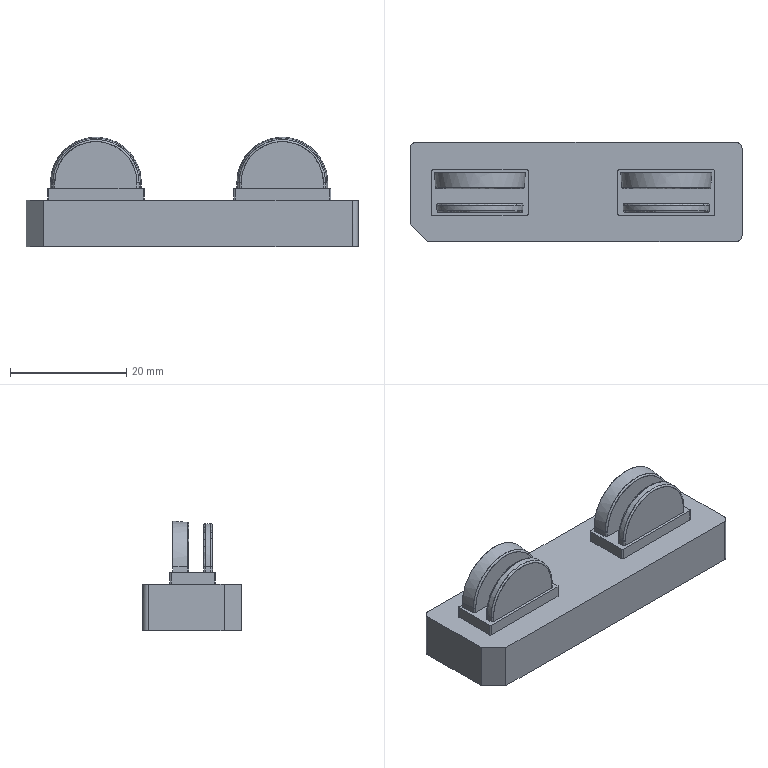NC program | PowerMill | posted by the shop | part box 57 x 17 x 18.807 mm
Lines 22103 to 22893 of 381081:
( TOOL ID   D10_1_1_1 )
( TOOL DIA. 10. TIP RAD 0 LENGTH 73.96 )
( Z = -11.01 )
T3 M6
T4
G91 G28 Z0
G0 G90 G54
M08
S8500 M3
X0 Y0 M8
G43 Z9.797 H3
X27.887 Y19.247
Z-9.81
G1 Z-11.01 F360
X27.699 Y13.975 F600
X18.085 Y9.168
X23.607
X23.828 Y9.163
X24.048 Y9.15
G2 X24.589 Y9.08 I-.615 J-6.925
G1 X24.858 Y9.026
G2 X26.347 Y8.449 I-1.315 J-5.601
G1 X26.555 Y8.325
G2 X27.127 Y7.914 I-3.108 J-4.931
G1 X27.189 Y7.865
X27.374 Y7.704
X27.552 Y7.534
X27.722 Y7.355
X27.884 Y7.17
X28.07 Y6.934
X28.211 Y6.738
X28.344 Y6.536
X28.467 Y6.329
X28.581 Y6.115
G2 X28.799 Y5.626 I-5.64 J-2.807
G1 X28.894 Y5.368
X28.976 Y5.106
X29.044 Y4.84
G2 X29.168 Y4.03 I-6.042 J-1.34
G1 X29.182 Y3.809
X29.187 Y3.588
Y-3.824
X29.182 Y-4.045
X29.168 Y-4.266
X29.14 Y-4.534
X29.099 Y-4.806
X29.044 Y-5.076
X28.976 Y-5.342
X28.894 Y-5.604
X28.78 Y-5.911
X28.685 Y-6.134
X28.581 Y-6.351
X28.467 Y-6.564
X28.344 Y-6.772
G2 X28.037 Y-7.214 I-5.063 J3.195
G1 X27.884 Y-7.406
X27.722 Y-7.592
G2 X27.374 Y-7.94 I-4.45 J4.102
G1 X27.189 Y-8.101
G2 X26.555 Y-8.561 I-3.982 J4.821
G1 X26.347 Y-8.685
X26.134 Y-8.799
X25.916 Y-8.903
G2 X25.387 Y-9.112 I-2.782 J6.274
G1 X25.124 Y-9.193
X24.858 Y-9.262
X24.589 Y-9.316
X24.268 Y-9.363
G2 X23.607 Y-9.404 I-.677 J5.595
G1 X7.393
G2 X6.527 Y-9.334 I.012 J5.527
G1 X6.411 Y-9.316
X6.142 Y-9.262
X5.876 Y-9.194
X5.613 Y-9.112
X5.306 Y-8.997
G2 X4.004 Y-8.254 I2.033 J5.076
G1 X3.811 Y-8.101
G2 X3.448 Y-7.77 I3.851 J4.585
X3.116 Y-7.406 I4.292 J4.249
X2.759 Y-6.929 I4.814 J3.975
G1 X2.656 Y-6.772
X2.539 Y-6.576
G2 X2.201 Y-5.862 I4.876 J2.751
G1 X2.106 Y-5.604
X2.024 Y-5.342
X1.956 Y-5.076
X1.901 Y-4.806
X1.86 Y-4.534
G2 X1.813 Y-3.824 I5.658 J.73
G1 Y3.588
X1.817 Y3.773
X1.838 Y4.104
X1.86 Y4.298
X1.901 Y4.57
X1.956 Y4.84
X2.024 Y5.106
X2.106 Y5.368
X2.22 Y5.675
X2.315 Y5.897
X2.419 Y6.116
X2.533 Y6.328
X2.656 Y6.536
G2 X2.97 Y6.987 I4.948 J-3.118
G1 X3.116 Y7.17
X3.278 Y7.356
X3.448 Y7.533
X3.626 Y7.704
G2 X4.033 Y8.04 I3.98 J-4.401
G1 X4.243 Y8.193
X4.445 Y8.325
X4.653 Y8.448
X4.866 Y8.563
X5.084 Y8.667
X5.27 Y8.746
X5.613 Y8.876
X5.876 Y8.958
X6.142 Y9.026
X6.411 Y9.08
X6.683 Y9.121
G2 X7.393 Y9.168 I.726 J-5.596
G1 X18.085
G0 Z2.804
G1 X1.885 Y4.466 F10000
G0 Z-10.91
G1 X1.86 Y4.298 Z-10.913 F360
X1.856 Y4.268
X1.854 Y4.25 Z-10.914
X1.827 Y3.959 Z-10.919
X1.813 Y3.588 Z-10.925
Y-1.26 Z-11.01
X-2.956 Y4.84 F600
X-2.901 Y4.57
X-2.854 Y4.25
X-2.832 Y4.03
X-2.818 Y3.809
X-2.813 Y3.588
Y-3.824
G2 X-2.854 Y-4.486 I-5.523 J.009
G1 X-2.901 Y-4.806
X-2.956 Y-5.076
X-3.024 Y-5.342
X-3.106 Y-5.604
X-3.22 Y-5.911
X-3.315 Y-6.134
X-3.419 Y-6.351
X-3.533 Y-6.564
X-3.656 Y-6.772
G2 X-3.963 Y-7.214 I-5.076 J3.204
G1 X-4.116 Y-7.406
X-4.278 Y-7.592
X-4.448 Y-7.769
X-4.626 Y-7.94
X-4.811 Y-8.101
G2 X-5.445 Y-8.561 I-4.018 J4.871
G1 X-5.653 Y-8.685
X-5.866 Y-8.798
X-6.084 Y-8.903
X-6.355 Y-9.017
X-6.613 Y-9.112
G2 X-7.142 Y-9.262 I-1.945 J5.846
G1 X-7.411 Y-9.316
X-7.683 Y-9.357
G2 X-8.172 Y-9.399 I-.745 J5.768
G1 X-8.393 Y-9.404
X-24.607
G2 X-25.95 Y-9.238 I.02 J5.69
G1 X-26.124 Y-9.193
G2 X-26.694 Y-8.997 I1.779 J6.081
G1 X-26.916 Y-8.903
G2 X-27.757 Y-8.429 I2.29 J5.043
G1 X-27.953 Y-8.287
G2 X-28.552 Y-7.77 I3.474 J4.631
G1 X-28.722 Y-7.592
G2 X-29.344 Y-6.772 I4.472 J4.038
G1 X-29.467 Y-6.564
X-29.581 Y-6.351
X-29.685 Y-6.134
X-29.793 Y-5.877
X-29.914 Y-5.542
X-29.976 Y-5.342
X-30.045 Y-5.075
X-30.099 Y-4.806
X-30.14 Y-4.534
G2 X-30.182 Y-4.045 I5.737 J.743
G1 X-30.187 Y-3.824
Y3.588
X-30.182 Y3.809
X-30.168 Y4.03
X-30.14 Y4.298
X-30.099 Y4.57
X-30.044 Y4.84
X-29.976 Y5.106
X-29.894 Y5.368
G2 X-29.685 Y5.898 I6.529 J-2.272
G1 X-29.581 Y6.115
X-29.467 Y6.329
X-29.343 Y6.536
X-29.211 Y6.738
G2 X-28.884 Y7.17 I5.641 J-3.936
G1 X-28.722 Y7.356
X-28.552 Y7.534
X-28.374 Y7.703
X-28.189 Y7.865
G2 X-27.555 Y8.325 I3.947 J-4.773
G1 X-27.347 Y8.449
X-27.134 Y8.562
X-26.916 Y8.667
X-26.645 Y8.781
X-26.387 Y8.876
G2 X-25.589 Y9.08 I1.818 J-5.43
G1 X-25.268 Y9.127
X-25.048 Y9.15
X-24.828 Y9.163
X-24.607 Y9.168
X-8.393
G2 X-7.079 Y9.01 I-.021 J-5.714
G1 X-6.876 Y8.957
G2 X-5.866 Y8.563 I-1.668 J-5.753
G1 X-5.653 Y8.449
X-5.445 Y8.325
G2 X-4.854 Y7.899 I-3.174 J-5.028
G1 X-4.626 Y7.704
X-4.448 Y7.534
X-4.278 Y7.356
X-4.116 Y7.17
X-3.93 Y6.934
X-3.789 Y6.738
X-3.656 Y6.536
G2 X-3.292 Y5.845 I-4.609 J-2.867
G1 X-3.201 Y5.626
X-3.106 Y5.368
X-3.024 Y5.106
X-2.956 Y4.84
G0 Z9.797
Z10.797
X0 Y0
X-4.092 Y-7.636
Z-9.78
G1 Z-10.98 F360
G3 X-5.2 Y-7.939 I-.188 J-1.488 F600
G2 X-8.306 Y-9.033 I-3.196 J4.117
G1 X-16.521 Y-9.034
X-24.555
G2 X-29.817 Y-3.834 I-.05 J5.212
G1 X-29.816 Y3.654
G2 X-24.554 Y8.798 I5.212 J-.068
G1 X-8.303 Y8.797
G2 X-3.184 Y3.651 I-.092 J-5.211
G1 X-3.183 Y-3.835
G2 X-5.2 Y-7.939 I-5.212 J.013
G3 X-5.768 Y-8.937 I.92 J-1.185
G1 X-4.16 Y-7.594
G3 X-5.269 Y-7.892 I-.195 J-1.487
G2 X-8.489 Y-8.954 I-3.128 J4.071
G1 X-16.521
X-24.554
X-24.555
G2 X-29.737 Y-3.834 I-.049 J5.132
G1 X-29.736 Y3.651
G2 X-24.554 Y8.718 I5.132 J-.065
G1 X-8.489
G2 X-3.264 Y3.651 I.091 J-5.133
G1 X-3.263 Y-3.834
G2 X-5.269 Y-7.892 I-5.134 J.013
G3 X-5.843 Y-8.886 I.914 J-1.189
G0 Z3.9
G1 X27.901 Y-7.644 F10000
G0 Z-9.78
G1 Z-10.98 F360
G3 X26.793 Y-7.945 I-.19 J-1.488 F600
G2 X23.641 Y-9.034 I-3.188 J4.123
G1 X7.392
G2 X2.268 Y-4.759 I.003 J5.211
G1 X2.251 Y-4.658
G2 X2.183 Y-3.834 I5.297 J.849
G1 Y-3.118
X2.184 Y3.654
G2 X7.394 Y8.798 I5.211 J-.067
G1 X23.643
G2 X28.816 Y3.651 I-.038 J-5.212
G1 X28.817 Y-3.835
G2 X26.793 Y-7.945 I-5.212 J.013
G3 X26.223 Y-8.942 I.918 J-1.187
G1 X27.833 Y-7.602
G3 X26.724 Y-7.898 I-.198 J-1.487
G2 X23.641 Y-8.954 I-3.119 J4.075
G1 X7.394
G2 X2.347 Y-4.746 I.001 J5.131
G1 X2.33 Y-4.645
G2 X2.263 Y-3.834 I5.216 J.836
G1 Y-3.118
X2.264 Y3.651
G2 X7.394 Y8.718 I5.131 J-.065
G1 X23.641
G2 X28.736 Y3.651 I-.036 J-5.132
G1 X28.737 Y-3.834
G2 X26.724 Y-7.898 I-5.132 J.011
G3 X26.148 Y-8.891 I.912 J-1.191
G0 Z10.797
X0 Y0
Z9.797
X32.183 Y-17.539
Z-17.71
G1 Z-18.91 F360
G3 X30.071 Y-13.007 I-1.056 J2.266 F600
G1 X29.91 Y-13.082
X29.907 Y-13.083
X29.905 Y-13.084
X29.589 Y-13.21
X29.587 Y-13.211
X29.585
X29.269 Y-13.317
X29.267
X29.266 Y-13.318
X29.139 Y-13.355
X29.138
X29.137 Y-13.356
X28.948 Y-13.405
X28.946 Y-13.406
X28.944
X28.628 Y-13.474
X28.626 Y-13.475
X28.624
X28.308 Y-13.526
X28.306
X28.303 Y-13.527
X27.987 Y-13.56
X27.985
X27.983
X27.667 Y-13.577
X27.665
X27.663
X27.347 Y-13.58
X-25.45
X-25.451
X-25.452
X-25.768 Y-13.573
X-25.77
X-25.773
X-26.089 Y-13.546
X-26.091 Y-13.545
X-26.094
X-26.41 Y-13.498
X-26.413 Y-13.497
X-26.415
X-26.731 Y-13.429
X-26.734 Y-13.428
X-26.736 Y-13.427
X-26.994 Y-13.355
X-26.997 Y-13.354
X-27.
X-27.373 Y-13.222
X-27.376 Y-13.221
X-27.379 Y-13.22
X-27.695 Y-13.081
X-27.696
X-27.698 Y-13.08
X-27.792 Y-13.034
X-27.793 Y-13.033
X-27.794 Y-13.032
X-28.017 Y-12.913
X-28.019 Y-12.911
X-28.021 Y-12.91
X-28.337 Y-12.714
X-28.34 Y-12.712
X-28.342 Y-12.71
X-28.658 Y-12.479
X-28.66 Y-12.477
X-28.662 Y-12.476
X-28.765 Y-12.392
X-28.766 Y-12.391
X-28.768 Y-12.389
X-28.98 Y-12.2
X-28.982 Y-12.199
X-28.983 Y-12.198
X-29.113 Y-12.071
X-29.114 Y-12.07
X-32.145 Y-9.038
X-32.146 Y-9.037
X-32.147 Y-9.036
X-32.268 Y-8.907
X-32.27 Y-8.905
X-32.271 Y-8.904
X-32.466 Y-8.675
X-32.467 Y-8.673
X-32.468 Y-8.672
X-32.536 Y-8.585
X-32.537 Y-8.584
X-32.538 Y-8.582
X-32.761 Y-8.266
X-32.763 Y-8.263
X-32.764 Y-8.261
X-32.953 Y-7.945
X-32.954 Y-7.942
X-32.956 Y-7.94
X-33.109 Y-7.637
X-33.11 Y-7.634
X-33.111 Y-7.632
X-33.249 Y-7.302
X-33.251 Y-7.3
Y-7.297
X-33.359 Y-6.981
X-33.36 Y-6.979
X-33.361 Y-6.976
X-33.43 Y-6.723
X-33.431 Y-6.721
X-33.432 Y-6.718
X-33.51 Y-6.339
X-33.511 Y-6.336
Y-6.334
X-33.554 Y-6.017
Y-6.015
Y-6.012
X-33.576 Y-5.696
Y-5.694
Y-5.692
X-33.58 Y-5.375
Y-5.374
X-33.579 Y7.588
Y7.589
Y7.591
X-33.566 Y7.907
Y7.909
Y7.911
X-33.536 Y8.227
Y8.229
Y8.231
X-33.489 Y8.548
Y8.55
X-33.488 Y8.552
X-33.432 Y8.834
X-33.431 Y8.836
Y8.838
X-33.341 Y9.188
X-33.34 Y9.19
Y9.193
X-33.238 Y9.509
Y9.511
X-33.237 Y9.513
X-33.116 Y9.829
X-33.115 Y9.831
X-33.114 Y9.833
X-32.972 Y10.149
X-32.971 Y10.152
X-32.97 Y10.154
X-32.805 Y10.47
X-32.804 Y10.472
X-32.803 Y10.474
X-32.613 Y10.79
X-32.612 Y10.792
X-32.61 Y10.794
X-32.471 Y11.
Y11.001
X-32.47 Y11.003
X-32.391 Y11.112
X-32.39 Y11.113
X-32.389 Y11.115
X-32.152 Y11.415
X-32.15 Y11.417
X-32.148 Y11.419
X-31.847 Y11.751
X-31.844 Y11.753
X-31.842 Y11.755
X-31.511 Y12.069
X-31.509 Y12.071
X-31.507 Y12.072
X-31.191 Y12.331
X-31.19 Y12.332
X-31.188 Y12.333
X-31.108 Y12.394
X-31.107 Y12.395
X-31.106
X-30.87 Y12.56
X-30.868 Y12.561
X-30.867 Y12.562
X-30.55 Y12.759
X-30.548 Y12.761
X-30.546 Y12.762
X-30.23 Y12.933
X-30.228 Y12.934
X-30.226 Y12.935
X-29.91 Y13.082
X-29.907 Y13.083
X-29.905 Y13.084
X-29.589 Y13.21
X-29.587 Y13.211
X-29.585
X-29.269 Y13.317
X-29.267 Y13.318
X-29.265
X-28.948 Y13.405
X-28.946
X-28.944 Y13.406
X-28.628 Y13.474
X-28.626 Y13.475
X-28.624
X-28.308 Y13.526
X-28.306
X-28.303 Y13.527
X-27.987 Y13.56
X-27.985
X-27.983
X-27.667 Y13.577
X-27.665
X-27.663
X-27.347 Y13.58
X0
X27.347
X27.663 Y13.577
X27.665
X27.667
X27.983 Y13.561
X27.985
X27.987 Y13.56
X28.304 Y13.527
X28.306 Y13.526
X28.308
X28.624 Y13.475
X28.626
X28.628 Y13.474
X28.944 Y13.406
X28.946 Y13.405
X28.948
X29.265 Y13.318
X29.267
X29.269 Y13.317
X29.585 Y13.211
X29.587 Y13.21
X29.589 Y13.209
X29.905 Y13.084
X29.907 Y13.083
X29.91 Y13.082
X30.226 Y12.934
X30.228 Y12.933
X30.23 Y12.932
X30.546 Y12.762
X30.548 Y12.761
X30.55 Y12.759
X30.866 Y12.563
X30.869 Y12.562
X30.871 Y12.56
X31.187 Y12.335
X31.189 Y12.333
X31.191 Y12.331
X31.504 Y12.075
X31.506 Y12.074
X31.508 Y12.072
X31.828 Y11.771
X31.83 Y11.768
X31.832 Y11.766
X32.134 Y11.435
X32.136 Y11.433
X32.138 Y11.431
X32.389 Y11.115
X32.39 Y11.113
X32.391 Y11.112
X32.47 Y11.002
X32.471 Y11.001
Y11.
X32.61 Y10.794
X32.611 Y10.792
X32.612 Y10.79
X32.79 Y10.498
X32.791 Y10.496
X32.792 Y10.494
X32.97 Y10.154
X32.971 Y10.152
X32.972 Y10.15
X33.11 Y9.844
X33.111 Y9.841
X33.112 Y9.839
X33.237 Y9.513
X33.238 Y9.511
Y9.509
X33.34 Y9.193
Y9.19
X33.341 Y9.188
X33.423 Y8.872
X33.424 Y8.87
Y8.868
X33.488 Y8.552
Y8.55
Y8.548
X33.536 Y8.232
Y8.229
Y8.227
X33.565 Y7.911
Y7.909
X33.566 Y7.907
X33.579 Y7.591
Y7.589
Y7.587
Y-7.587
Y-7.589
Y-7.591
X33.566 Y-7.907
Y-7.909
Y-7.911
X33.536 Y-8.227
Y-8.229
Y-8.231
X33.489 Y-8.548
Y-8.55
X33.488 Y-8.552
X33.432 Y-8.834
X33.431 Y-8.836
Y-8.838
X33.341 Y-9.188
X33.34 Y-9.19
Y-9.193
X33.238 Y-9.509
Y-9.511
X33.237 Y-9.513
X33.116 Y-9.829
X33.115 Y-9.831
X33.114 Y-9.833
X32.972 Y-10.149
X32.971 Y-10.152
X32.97 Y-10.154
X32.805 Y-10.47
X32.804 Y-10.472
X32.803 Y-10.474
X32.613 Y-10.79
X32.612 Y-10.792
X32.61 Y-10.794
X32.471 Y-11.
Y-11.001
X32.47 Y-11.003
X32.391 Y-11.112
X32.39 Y-11.113
X32.389 Y-11.115
X32.152 Y-11.415
X32.15 Y-11.417
X32.148 Y-11.419
X31.847 Y-11.751
X31.844 Y-11.753
X31.842 Y-11.755
X31.511 Y-12.069
X31.509 Y-12.071
X31.507 Y-12.072
X31.191 Y-12.331
X31.19 Y-12.332
X31.188 Y-12.333
X31.108 Y-12.394
X31.107 Y-12.395
X31.106
X30.87 Y-12.56
X30.868 Y-12.561
X30.867 Y-12.562
X30.55 Y-12.759
X30.548 Y-12.761
X30.546 Y-12.762
X30.23 Y-12.933
X30.228 Y-12.934
X30.226 Y-12.935
X30.071 Y-13.007
G3 X32.183 Y-17.539 I1.056 J-2.266
G1 X32.136 Y-17.472
G3 X30.025 Y-12.94 I-1.056 J2.266
G1 X29.876 Y-13.01
X29.56 Y-13.135
X29.243 Y-13.241
X29.116 Y-13.278
X28.927 Y-13.328
X28.611 Y-13.396
X28.295 Y-13.447
X27.979 Y-13.481
X27.663 Y-13.497
X27.347 Y-13.5
X-25.45
X-25.766 Y-13.493
X-26.082 Y-13.466
X-26.398 Y-13.419
X-26.714 Y-13.35
X-26.973 Y-13.278
X-27.347 Y-13.147
X-27.663 Y-13.008
X-27.756 Y-12.962
X-27.979 Y-12.842
X-28.295 Y-12.646
X-28.611 Y-12.414
X-28.715 Y-12.33
X-28.927 Y-12.141
X-29.058 Y-12.014
X-32.089 Y-8.981
X-32.21 Y-8.852
X-32.405 Y-8.623
X-32.473 Y-8.536
X-32.696 Y-8.22
X-32.884 Y-7.904
X-33.037 Y-7.601
X-33.176 Y-7.271
X-33.284 Y-6.955
X-33.353 Y-6.702
X-33.432 Y-6.323
X-33.474 Y-6.007
X-33.496 Y-5.691
X-33.5 Y-5.374
Y7.271
X-33.499 Y7.587
X-33.486 Y7.904
X-33.457 Y8.22
X-33.41 Y8.536
X-33.353 Y8.818
X-33.263 Y9.168
X-33.162 Y9.484
X-33.041 Y9.801
X-32.899 Y10.117
X-32.734 Y10.433
X-32.544 Y10.749
X-32.405 Y10.956
X-32.326 Y11.065
X-32.089 Y11.366
X-31.787 Y11.697
X-31.456 Y12.011
X-31.14 Y12.269
X-31.06 Y12.33
X-30.824 Y12.494
X-30.508 Y12.692
X-30.192 Y12.862
X-29.876 Y13.01
X-29.56 Y13.135
X-29.243 Y13.241
X-28.927 Y13.328
X-28.611 Y13.396
X-28.295 Y13.447
X-27.979 Y13.481
X-27.663 Y13.497
X-27.347 Y13.5
X0
X27.347
X27.663 Y13.497
X27.979 Y13.481
X28.295 Y13.447
X28.611 Y13.396
X28.927 Y13.328
X29.243 Y13.241
X29.56 Y13.135
X29.876 Y13.01
X30.192 Y12.862
X30.508 Y12.692
X30.824 Y12.495
X31.14 Y12.269
X31.453 Y12.014
X31.773 Y11.712
X32.075 Y11.381
X32.326 Y11.065
X32.405 Y10.955
X32.544 Y10.749
X32.721 Y10.456
X32.899 Y10.117
X33.037 Y9.811
X33.162 Y9.484
X33.263 Y9.168
X33.346 Y8.852
X33.409 Y8.536
X33.457 Y8.22
X33.486 Y7.904
X33.499 Y7.587
X33.5 Y7.271
Y-7.271
X33.499 Y-7.587
X33.486 Y-7.904
X33.457 Y-8.22
X33.41 Y-8.536
X33.353 Y-8.818
X33.263 Y-9.168
X33.162 Y-9.484
X33.041 Y-9.801
X32.899 Y-10.117
X32.734 Y-10.433
X32.544 Y-10.749
X32.405 Y-10.956
X32.326 Y-11.065
X32.089 Y-11.366
X31.787 Y-11.697
X31.456 Y-12.011
X31.14 Y-12.269
X31.06 Y-12.33
X30.824 Y-12.494
X30.508 Y-12.692
X30.192 Y-12.862
X30.025 Y-12.94
G3 X32.136 Y-17.472 I1.056 J-2.266
G0 Z9.797
Z10.797
X0 Y0
M9
M5
M01